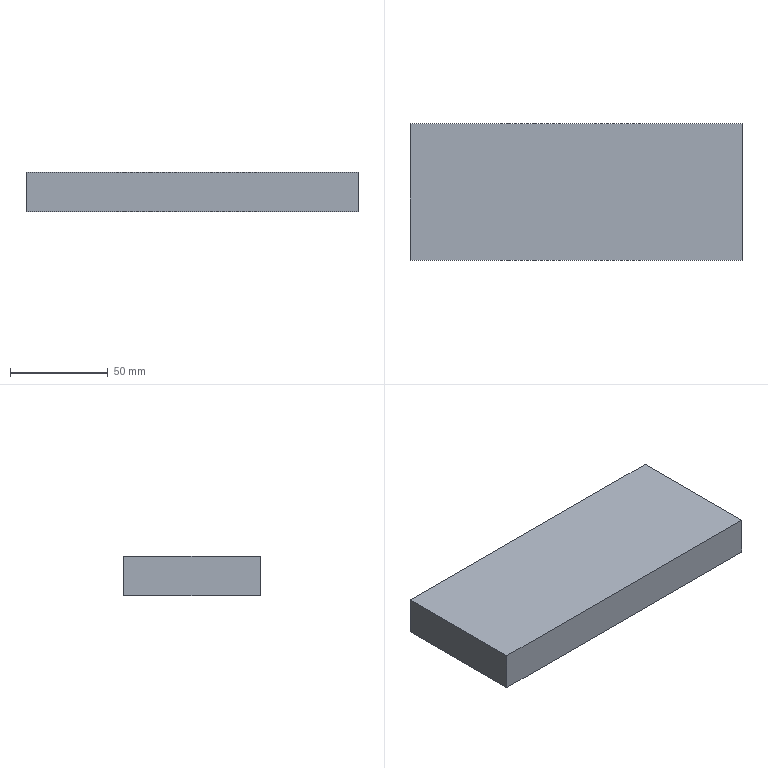Part | SolidWorks | features Extrusion 1 | 1 solid | 6 faces | box 170 x 70 x 20 mm | volume 238000 mm3 | plane 6
STEP:
#1=CARTESIAN_POINT('',(-85.,35.,0.));
#2=VERTEX_POINT('',#1);
#3=CARTESIAN_POINT('',(-85.,-35.,0.));
#4=VERTEX_POINT('',#3);
#5=CARTESIAN_POINT('',(-85.,35.,0.));
#6=DIRECTION('',(0.,-1.,0.));
#7=VECTOR('',#6,1000.);
#8=LINE('',#5,#7);
#9=EDGE_CURVE('',#2,#4,#8,.T.);
#10=ORIENTED_EDGE('',*,*,#9,.T.);
#11=CARTESIAN_POINT('',(-85.,-35.,20.));
#12=VERTEX_POINT('',#11);
#13=CARTESIAN_POINT('',(-85.,-35.,20.));
#14=DIRECTION('',(0.,0.,-1.));
#15=VECTOR('',#14,1000.);
#16=LINE('',#13,#15);
#17=EDGE_CURVE('',#12,#4,#16,.T.);
#18=ORIENTED_EDGE('',*,*,#17,.F.);
#19=CARTESIAN_POINT('',(-85.,35.,20.));
#20=VERTEX_POINT('',#19);
#21=CARTESIAN_POINT('',(-85.,35.,20.));
#22=DIRECTION('',(0.,-1.,0.));
#23=VECTOR('',#22,1000.);
#24=LINE('',#21,#23);
#25=EDGE_CURVE('',#20,#12,#24,.T.);
#26=ORIENTED_EDGE('',*,*,#25,.F.);
#27=CARTESIAN_POINT('',(-85.,35.,20.));
#28=DIRECTION('',(0.,0.,-1.));
#29=VECTOR('',#28,1000.);
#30=LINE('',#27,#29);
#31=EDGE_CURVE('',#20,#2,#30,.T.);
#32=ORIENTED_EDGE('',*,*,#31,.T.);
#33=EDGE_LOOP('',(#10,#18,#26,#32));
#34=FACE_OUTER_BOUND('',#33,.T.);
#35=CARTESIAN_POINT('',(-85.,35.,20.));
#36=DIRECTION('',(1.,0.,0.));
#37=DIRECTION('',(0.,0.,-1.));
#38=AXIS2_PLACEMENT_3D('',#35,#36,#37);
#39=PLANE('',#38);
#40=ADVANCED_FACE('',(#34),#39,.F.);
#41=CARTESIAN_POINT('',(85.,-35.,0.));
#42=VERTEX_POINT('',#41);
#43=CARTESIAN_POINT('',(85.,-35.,0.));
#44=DIRECTION('',(1.,0.,0.));
#45=VECTOR('',#44,1000.);
#46=LINE('',#43,#45);
#47=EDGE_CURVE('',#4,#42,#46,.T.);
#48=ORIENTED_EDGE('',*,*,#47,.T.);
#49=CARTESIAN_POINT('',(85.,-35.,20.));
#50=VERTEX_POINT('',#49);
#51=CARTESIAN_POINT('',(85.,-35.,20.));
#52=DIRECTION('',(0.,0.,-1.));
#53=VECTOR('',#52,1000.);
#54=LINE('',#51,#53);
#55=EDGE_CURVE('',#50,#42,#54,.T.);
#56=ORIENTED_EDGE('',*,*,#55,.F.);
#57=CARTESIAN_POINT('',(85.,-35.,20.));
#58=DIRECTION('',(1.,0.,0.));
#59=VECTOR('',#58,1000.);
#60=LINE('',#57,#59);
#61=EDGE_CURVE('',#12,#50,#60,.T.);
#62=ORIENTED_EDGE('',*,*,#61,.F.);
#63=ORIENTED_EDGE('',*,*,#17,.T.);
#64=EDGE_LOOP('',(#48,#56,#62,#63));
#65=FACE_OUTER_BOUND('',#64,.T.);
#66=CARTESIAN_POINT('',(85.,-35.,20.));
#67=DIRECTION('',(0.,1.,0.));
#68=DIRECTION('',(-1.,0.,0.));
#69=AXIS2_PLACEMENT_3D('',#66,#67,#68);
#70=PLANE('',#69);
#71=ADVANCED_FACE('',(#65),#70,.F.);
#72=CARTESIAN_POINT('',(85.,35.,0.));
#73=VERTEX_POINT('',#72);
#74=CARTESIAN_POINT('',(85.,35.,0.));
#75=DIRECTION('',(0.,1.,0.));
#76=VECTOR('',#75,1000.);
#77=LINE('',#74,#76);
#78=EDGE_CURVE('',#42,#73,#77,.T.);
#79=ORIENTED_EDGE('',*,*,#78,.T.);
#80=CARTESIAN_POINT('',(85.,35.,20.));
#81=VERTEX_POINT('',#80);
#82=CARTESIAN_POINT('',(85.,35.,20.));
#83=DIRECTION('',(0.,0.,-1.));
#84=VECTOR('',#83,1000.);
#85=LINE('',#82,#84);
#86=EDGE_CURVE('',#81,#73,#85,.T.);
#87=ORIENTED_EDGE('',*,*,#86,.F.);
#88=CARTESIAN_POINT('',(85.,35.,20.));
#89=DIRECTION('',(0.,1.,0.));
#90=VECTOR('',#89,1000.);
#91=LINE('',#88,#90);
#92=EDGE_CURVE('',#50,#81,#91,.T.);
#93=ORIENTED_EDGE('',*,*,#92,.F.);
#94=ORIENTED_EDGE('',*,*,#55,.T.);
#95=EDGE_LOOP('',(#79,#87,#93,#94));
#96=FACE_OUTER_BOUND('',#95,.T.);
#97=CARTESIAN_POINT('',(85.,35.,20.));
#98=DIRECTION('',(-1.,0.,0.));
#99=DIRECTION('',(0.,-1.,0.));
#100=AXIS2_PLACEMENT_3D('',#97,#98,#99);
#101=PLANE('',#100);
#102=ADVANCED_FACE('',(#96),#101,.F.);
#103=CARTESIAN_POINT('',(85.,35.,0.));
#104=DIRECTION('',(-1.,0.,0.));
#105=VECTOR('',#104,1000.);
#106=LINE('',#103,#105);
#107=EDGE_CURVE('',#73,#2,#106,.T.);
#108=ORIENTED_EDGE('',*,*,#107,.T.);
#109=ORIENTED_EDGE('',*,*,#31,.F.);
#110=CARTESIAN_POINT('',(85.,35.,20.));
#111=DIRECTION('',(-1.,0.,0.));
#112=VECTOR('',#111,1000.);
#113=LINE('',#110,#112);
#114=EDGE_CURVE('',#81,#20,#113,.T.);
#115=ORIENTED_EDGE('',*,*,#114,.F.);
#116=ORIENTED_EDGE('',*,*,#86,.T.);
#117=EDGE_LOOP('',(#108,#109,#115,#116));
#118=FACE_OUTER_BOUND('',#117,.T.);
#119=CARTESIAN_POINT('',(85.,35.,20.));
#120=DIRECTION('',(0.,-1.,0.));
#121=DIRECTION('',(1.,0.,0.));
#122=AXIS2_PLACEMENT_3D('',#119,#120,#121);
#123=PLANE('',#122);
#124=ADVANCED_FACE('',(#118),#123,.F.);
#125=ORIENTED_EDGE('',*,*,#25,.T.);
#126=ORIENTED_EDGE('',*,*,#61,.T.);
#127=ORIENTED_EDGE('',*,*,#92,.T.);
#128=ORIENTED_EDGE('',*,*,#114,.T.);
#129=EDGE_LOOP('',(#125,#126,#127,#128));
#130=FACE_OUTER_BOUND('',#129,.T.);
#131=CARTESIAN_POINT('',(0.,0.,20.));
#132=DIRECTION('',(0.,0.,-1.));
#133=DIRECTION('',(-1.,0.,0.));
#134=AXIS2_PLACEMENT_3D('',#131,#132,#133);
#135=PLANE('',#134);
#136=ADVANCED_FACE('',(#130),#135,.F.);
#137=ORIENTED_EDGE('',*,*,#9,.F.);
#138=ORIENTED_EDGE('',*,*,#107,.F.);
#139=ORIENTED_EDGE('',*,*,#78,.F.);
#140=ORIENTED_EDGE('',*,*,#47,.F.);
#141=EDGE_LOOP('',(#137,#138,#139,#140));
#142=FACE_OUTER_BOUND('',#141,.T.);
#143=CARTESIAN_POINT('',(0.,0.,0.));
#144=DIRECTION('',(0.,0.,-1.));
#145=DIRECTION('',(-1.,0.,0.));
#146=AXIS2_PLACEMENT_3D('',#143,#144,#145);
#147=PLANE('',#146);
#148=ADVANCED_FACE('',(#142),#147,.T.);
#149=CLOSED_SHELL('',(#40,#71,#102,#124,#136,#148));
#150=MANIFOLD_SOLID_BREP('',#149);
#151=CARTESIAN_POINT('',(0.,0.,0.));
#152=DIRECTION('',(0.,0.,1.));
#153=DIRECTION('',(1.,0.,0.));
#154=AXIS2_PLACEMENT_3D('',#151,#152,#153);
#155=(LENGTH_UNIT()NAMED_UNIT(*)SI_UNIT(.MILLI.,.METRE.));
#156=UNCERTAINTY_MEASURE_WITH_UNIT(LENGTH_MEASURE(0.00001),#155,'','');
#157=(NAMED_UNIT(*)PLANE_ANGLE_UNIT()SI_UNIT($,.RADIAN.));
#158=(NAMED_UNIT(*)SI_UNIT($,.STERADIAN.)SOLID_ANGLE_UNIT());
#159=(GEOMETRIC_REPRESENTATION_CONTEXT(3)GLOBAL_UNCERTAINTY_ASSIGNED_CONTEXT((#156))GLOBAL_UNIT_ASSIGNED_CONTEXT((#155,#157,#158))REPRESENTATION_CONTEXT('',''));
#160=ADVANCED_BREP_SHAPE_REPRESENTATION('',(#150,#154),#159);